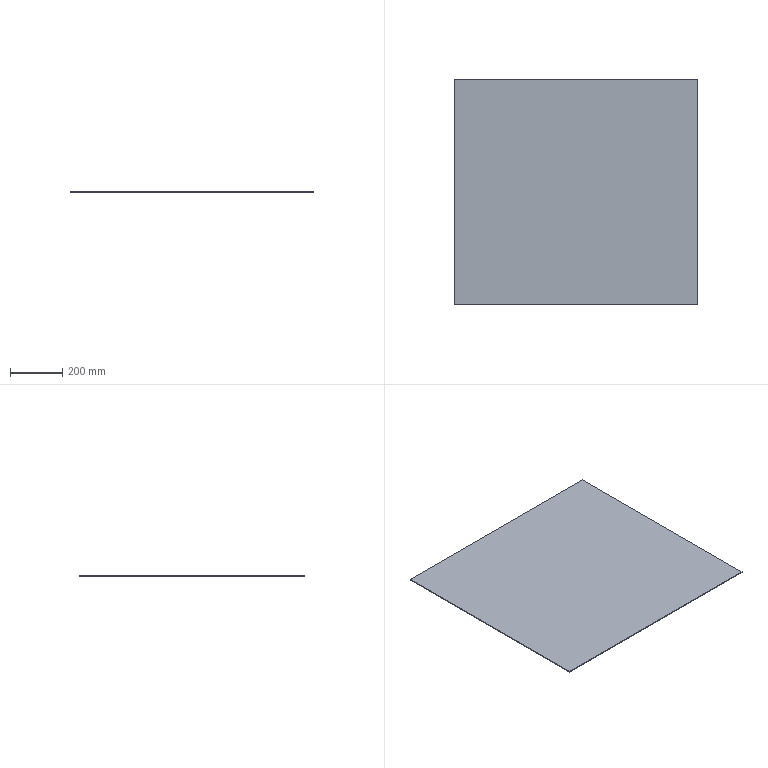Part | 1 solid | 6 faces | box 935 x 865 x 3 mm | volume 2426325 mm3 | plane 6
STEP:
#1=CARTESIAN_POINT('',(467.5,-432.5,0.));
#2=VERTEX_POINT('',#1);
#3=CARTESIAN_POINT('',(467.5,432.5,0.));
#4=VERTEX_POINT('',#3);
#5=CARTESIAN_POINT('',(467.5,432.5,0.));
#6=DIRECTION('',(0.,1.,0.));
#7=VECTOR('',#6,1000.);
#8=LINE('',#5,#7);
#9=EDGE_CURVE('',#2,#4,#8,.T.);
#10=ORIENTED_EDGE('',*,*,#9,.T.);
#11=CARTESIAN_POINT('',(467.5,432.5,3.));
#12=VERTEX_POINT('',#11);
#13=CARTESIAN_POINT('',(467.5,432.5,3.));
#14=DIRECTION('',(0.,0.,-1.));
#15=VECTOR('',#14,1000.);
#16=LINE('',#13,#15);
#17=EDGE_CURVE('',#12,#4,#16,.T.);
#18=ORIENTED_EDGE('',*,*,#17,.F.);
#19=CARTESIAN_POINT('',(467.5,-432.5,3.));
#20=VERTEX_POINT('',#19);
#21=CARTESIAN_POINT('',(467.5,432.5,3.));
#22=DIRECTION('',(0.,1.,0.));
#23=VECTOR('',#22,1000.);
#24=LINE('',#21,#23);
#25=EDGE_CURVE('',#20,#12,#24,.T.);
#26=ORIENTED_EDGE('',*,*,#25,.F.);
#27=CARTESIAN_POINT('',(467.5,-432.5,3.));
#28=DIRECTION('',(0.,0.,-1.));
#29=VECTOR('',#28,1000.);
#30=LINE('',#27,#29);
#31=EDGE_CURVE('',#20,#2,#30,.T.);
#32=ORIENTED_EDGE('',*,*,#31,.T.);
#33=EDGE_LOOP('',(#10,#18,#26,#32));
#34=FACE_OUTER_BOUND('',#33,.T.);
#35=CARTESIAN_POINT('',(467.5,432.5,3.));
#36=DIRECTION('',(-1.,0.,0.));
#37=DIRECTION('',(0.,-1.,0.));
#38=AXIS2_PLACEMENT_3D('',#35,#36,#37);
#39=PLANE('',#38);
#40=ADVANCED_FACE('',(#34),#39,.F.);
#41=CARTESIAN_POINT('',(-467.5,432.5,0.));
#42=VERTEX_POINT('',#41);
#43=CARTESIAN_POINT('',(-467.5,432.5,0.));
#44=DIRECTION('',(-1.,0.,0.));
#45=VECTOR('',#44,1000.);
#46=LINE('',#43,#45);
#47=EDGE_CURVE('',#4,#42,#46,.T.);
#48=ORIENTED_EDGE('',*,*,#47,.T.);
#49=CARTESIAN_POINT('',(-467.5,432.5,3.));
#50=VERTEX_POINT('',#49);
#51=CARTESIAN_POINT('',(-467.5,432.5,3.));
#52=DIRECTION('',(0.,0.,-1.));
#53=VECTOR('',#52,1000.);
#54=LINE('',#51,#53);
#55=EDGE_CURVE('',#50,#42,#54,.T.);
#56=ORIENTED_EDGE('',*,*,#55,.F.);
#57=CARTESIAN_POINT('',(-467.5,432.5,3.));
#58=DIRECTION('',(-1.,0.,0.));
#59=VECTOR('',#58,1000.);
#60=LINE('',#57,#59);
#61=EDGE_CURVE('',#12,#50,#60,.T.);
#62=ORIENTED_EDGE('',*,*,#61,.F.);
#63=ORIENTED_EDGE('',*,*,#17,.T.);
#64=EDGE_LOOP('',(#48,#56,#62,#63));
#65=FACE_OUTER_BOUND('',#64,.T.);
#66=CARTESIAN_POINT('',(-467.5,432.5,3.));
#67=DIRECTION('',(0.,-1.,0.));
#68=DIRECTION('',(0.,0.,-1.));
#69=AXIS2_PLACEMENT_3D('',#66,#67,#68);
#70=PLANE('',#69);
#71=ADVANCED_FACE('',(#65),#70,.F.);
#72=CARTESIAN_POINT('',(-467.5,-432.5,0.));
#73=VERTEX_POINT('',#72);
#74=CARTESIAN_POINT('',(-467.5,432.5,0.));
#75=DIRECTION('',(0.,-1.,0.));
#76=VECTOR('',#75,1000.);
#77=LINE('',#74,#76);
#78=EDGE_CURVE('',#42,#73,#77,.T.);
#79=ORIENTED_EDGE('',*,*,#78,.T.);
#80=CARTESIAN_POINT('',(-467.5,-432.5,3.));
#81=VERTEX_POINT('',#80);
#82=CARTESIAN_POINT('',(-467.5,-432.5,3.));
#83=DIRECTION('',(0.,0.,-1.));
#84=VECTOR('',#83,1000.);
#85=LINE('',#82,#84);
#86=EDGE_CURVE('',#81,#73,#85,.T.);
#87=ORIENTED_EDGE('',*,*,#86,.F.);
#88=CARTESIAN_POINT('',(-467.5,432.5,3.));
#89=DIRECTION('',(0.,-1.,0.));
#90=VECTOR('',#89,1000.);
#91=LINE('',#88,#90);
#92=EDGE_CURVE('',#50,#81,#91,.T.);
#93=ORIENTED_EDGE('',*,*,#92,.F.);
#94=ORIENTED_EDGE('',*,*,#55,.T.);
#95=EDGE_LOOP('',(#79,#87,#93,#94));
#96=FACE_OUTER_BOUND('',#95,.T.);
#97=CARTESIAN_POINT('',(-467.5,432.5,3.));
#98=DIRECTION('',(1.,0.,0.));
#99=DIRECTION('',(0.,1.,0.));
#100=AXIS2_PLACEMENT_3D('',#97,#98,#99);
#101=PLANE('',#100);
#102=ADVANCED_FACE('',(#96),#101,.F.);
#103=CARTESIAN_POINT('',(-467.5,-432.5,0.));
#104=DIRECTION('',(1.,0.,0.));
#105=VECTOR('',#104,1000.);
#106=LINE('',#103,#105);
#107=EDGE_CURVE('',#73,#2,#106,.T.);
#108=ORIENTED_EDGE('',*,*,#107,.T.);
#109=ORIENTED_EDGE('',*,*,#31,.F.);
#110=CARTESIAN_POINT('',(-467.5,-432.5,3.));
#111=DIRECTION('',(1.,0.,0.));
#112=VECTOR('',#111,1000.);
#113=LINE('',#110,#112);
#114=EDGE_CURVE('',#81,#20,#113,.T.);
#115=ORIENTED_EDGE('',*,*,#114,.F.);
#116=ORIENTED_EDGE('',*,*,#86,.T.);
#117=EDGE_LOOP('',(#108,#109,#115,#116));
#118=FACE_OUTER_BOUND('',#117,.T.);
#119=CARTESIAN_POINT('',(-467.5,-432.5,3.));
#120=DIRECTION('',(0.,1.,0.));
#121=DIRECTION('',(0.,0.,1.));
#122=AXIS2_PLACEMENT_3D('',#119,#120,#121);
#123=PLANE('',#122);
#124=ADVANCED_FACE('',(#118),#123,.F.);
#125=ORIENTED_EDGE('',*,*,#25,.T.);
#126=ORIENTED_EDGE('',*,*,#61,.T.);
#127=ORIENTED_EDGE('',*,*,#92,.T.);
#128=ORIENTED_EDGE('',*,*,#114,.T.);
#129=EDGE_LOOP('',(#125,#126,#127,#128));
#130=FACE_OUTER_BOUND('',#129,.T.);
#131=CARTESIAN_POINT('',(0.,0.,3.));
#132=DIRECTION('',(0.,0.,1.));
#133=DIRECTION('',(1.,0.,0.));
#134=AXIS2_PLACEMENT_3D('',#131,#132,#133);
#135=PLANE('',#134);
#136=ADVANCED_FACE('',(#130),#135,.T.);
#137=ORIENTED_EDGE('',*,*,#9,.F.);
#138=ORIENTED_EDGE('',*,*,#107,.F.);
#139=ORIENTED_EDGE('',*,*,#78,.F.);
#140=ORIENTED_EDGE('',*,*,#47,.F.);
#141=EDGE_LOOP('',(#137,#138,#139,#140));
#142=FACE_OUTER_BOUND('',#141,.T.);
#143=CARTESIAN_POINT('',(0.,0.,0.));
#144=DIRECTION('',(0.,0.,1.));
#145=DIRECTION('',(1.,0.,0.));
#146=AXIS2_PLACEMENT_3D('',#143,#144,#145);
#147=PLANE('',#146);
#148=ADVANCED_FACE('',(#142),#147,.F.);
#149=CLOSED_SHELL('',(#40,#71,#102,#124,#136,#148));
#150=MANIFOLD_SOLID_BREP('',#149);
#151=CARTESIAN_POINT('',(0.,0.,0.));
#152=DIRECTION('',(0.,0.,1.));
#153=DIRECTION('',(1.,0.,0.));
#154=AXIS2_PLACEMENT_3D('',#151,#152,#153);
#155=(LENGTH_UNIT()NAMED_UNIT(*)SI_UNIT(.MILLI.,.METRE.));
#156=UNCERTAINTY_MEASURE_WITH_UNIT(LENGTH_MEASURE(0.00001),#155,'','');
#157=(NAMED_UNIT(*)PLANE_ANGLE_UNIT()SI_UNIT($,.RADIAN.));
#158=(NAMED_UNIT(*)SI_UNIT($,.STERADIAN.)SOLID_ANGLE_UNIT());
#159=(GEOMETRIC_REPRESENTATION_CONTEXT(3)GLOBAL_UNCERTAINTY_ASSIGNED_CONTEXT((#156))GLOBAL_UNIT_ASSIGNED_CONTEXT((#155,#157,#158))REPRESENTATION_CONTEXT('',''));
#160=ADVANCED_BREP_SHAPE_REPRESENTATION('',(#150,#154),#159);